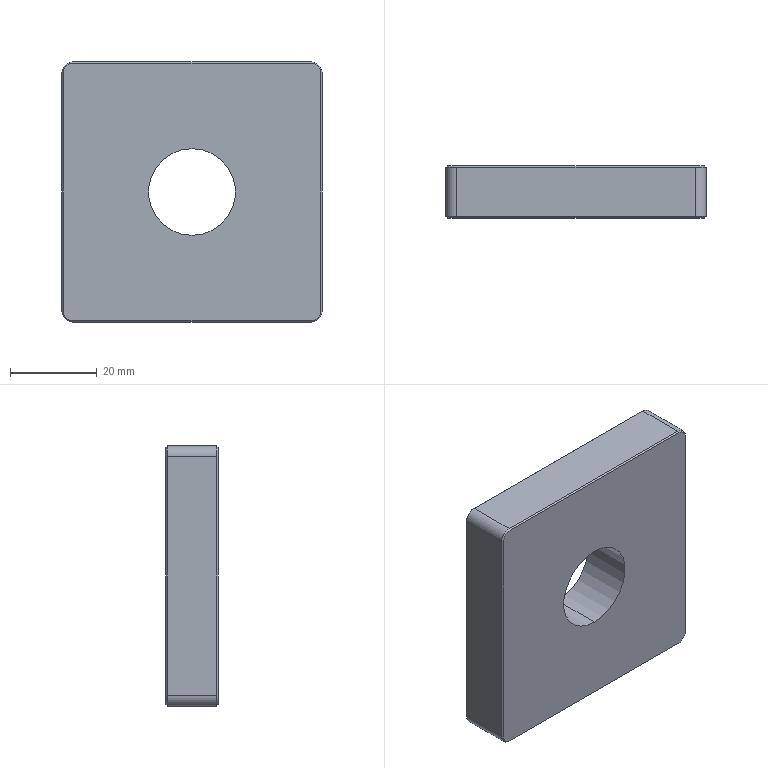Part | SolidWorks | features BaseBody 1 | 1 solid | 28 faces | box 60 x 12 x 60 mm | volume 39345 mm3 | plane 14 | cone 8 | cylinder 6 | commonest cylinder face diameters 5 x4 20 x2
STEP:
#1=CARTESIAN_POINT('',(0.,6.,-10.));
#2=VERTEX_POINT('',#1);
#3=CARTESIAN_POINT('',(0.,6.,10.));
#4=VERTEX_POINT('',#3);
#5=CARTESIAN_POINT('',(0.,6.,0.));
#6=DIRECTION('',(0.,1.,0.));
#7=DIRECTION('',(0.,0.,-1.));
#8=AXIS2_PLACEMENT_3D('',#5,#6,#7);
#9=CIRCLE('',#8,10.);
#10=EDGE_CURVE('',#2,#4,#9,.T.);
#11=ORIENTED_EDGE('',*,*,#10,.T.);
#12=CARTESIAN_POINT('',(0.,-6.,10.));
#13=VERTEX_POINT('',#12);
#14=CARTESIAN_POINT('',(0.,6.,10.));
#15=DIRECTION('',(0.,-1.,0.));
#16=VECTOR('',#15,1000.);
#17=LINE('',#14,#16);
#18=EDGE_CURVE('',#4,#13,#17,.T.);
#19=ORIENTED_EDGE('',*,*,#18,.T.);
#20=CARTESIAN_POINT('',(0.,-6.,-10.));
#21=VERTEX_POINT('',#20);
#22=CARTESIAN_POINT('',(0.,-6.,0.));
#23=DIRECTION('',(0.,1.,0.));
#24=DIRECTION('',(0.,0.,-1.));
#25=AXIS2_PLACEMENT_3D('',#22,#23,#24);
#26=CIRCLE('',#25,10.);
#27=EDGE_CURVE('',#21,#13,#26,.T.);
#28=ORIENTED_EDGE('',*,*,#27,.F.);
#29=CARTESIAN_POINT('',(0.,6.,-10.));
#30=DIRECTION('',(0.,-1.,0.));
#31=VECTOR('',#30,1000.);
#32=LINE('',#29,#31);
#33=EDGE_CURVE('',#2,#21,#32,.T.);
#34=ORIENTED_EDGE('',*,*,#33,.F.);
#35=EDGE_LOOP('',(#11,#19,#28,#34));
#36=FACE_OUTER_BOUND('',#35,.T.);
#37=CARTESIAN_POINT('',(0.,6.,0.));
#38=DIRECTION('',(0.,-1.,0.));
#39=DIRECTION('',(0.,0.,-1.));
#40=AXIS2_PLACEMENT_3D('',#37,#38,#39);
#41=CYLINDRICAL_SURFACE('',#40,10.);
#42=ADVANCED_FACE('',(#36),#41,.F.);
#43=CARTESIAN_POINT('',(-27.5,6.,-29.7));
#44=VERTEX_POINT('',#43);
#45=CARTESIAN_POINT('',(27.5,6.,-29.7));
#46=VERTEX_POINT('',#45);
#47=CARTESIAN_POINT('',(0.,6.,-29.7));
#48=DIRECTION('',(1.,0.,0.));
#49=VECTOR('',#48,1000.);
#50=LINE('',#47,#49);
#51=EDGE_CURVE('',#44,#46,#50,.T.);
#52=ORIENTED_EDGE('',*,*,#51,.F.);
#53=CARTESIAN_POINT('',(-29.7,6.,-27.5));
#54=VERTEX_POINT('',#53);
#55=CARTESIAN_POINT('',(-27.5,6.,-27.5));
#56=DIRECTION('',(0.,-1.,0.));
#57=DIRECTION('',(0.,0.,-1.));
#58=AXIS2_PLACEMENT_3D('',#55,#56,#57);
#59=CIRCLE('',#58,2.2);
#60=EDGE_CURVE('',#54,#44,#59,.T.);
#61=ORIENTED_EDGE('',*,*,#60,.F.);
#62=CARTESIAN_POINT('',(-29.7,6.,27.5));
#63=VERTEX_POINT('',#62);
#64=CARTESIAN_POINT('',(-29.7,6.,0.));
#65=DIRECTION('',(0.,0.,-1.));
#66=VECTOR('',#65,1000.);
#67=LINE('',#64,#66);
#68=EDGE_CURVE('',#63,#54,#67,.T.);
#69=ORIENTED_EDGE('',*,*,#68,.F.);
#70=CARTESIAN_POINT('',(-27.5,6.,29.7));
#71=VERTEX_POINT('',#70);
#72=CARTESIAN_POINT('',(-27.5,6.,27.5));
#73=DIRECTION('',(0.,-1.,0.));
#74=DIRECTION('',(0.,0.,-1.));
#75=AXIS2_PLACEMENT_3D('',#72,#73,#74);
#76=CIRCLE('',#75,2.2);
#77=EDGE_CURVE('',#71,#63,#76,.T.);
#78=ORIENTED_EDGE('',*,*,#77,.F.);
#79=CARTESIAN_POINT('',(27.5,6.,29.7));
#80=VERTEX_POINT('',#79);
#81=CARTESIAN_POINT('',(0.,6.,29.7));
#82=DIRECTION('',(-1.,0.,0.));
#83=VECTOR('',#82,1000.);
#84=LINE('',#81,#83);
#85=EDGE_CURVE('',#80,#71,#84,.T.);
#86=ORIENTED_EDGE('',*,*,#85,.F.);
#87=CARTESIAN_POINT('',(29.7,6.,27.5));
#88=VERTEX_POINT('',#87);
#89=CARTESIAN_POINT('',(27.5,6.,27.5));
#90=DIRECTION('',(0.,-1.,0.));
#91=DIRECTION('',(0.,0.,-1.));
#92=AXIS2_PLACEMENT_3D('',#89,#90,#91);
#93=CIRCLE('',#92,2.2);
#94=EDGE_CURVE('',#88,#80,#93,.T.);
#95=ORIENTED_EDGE('',*,*,#94,.F.);
#96=CARTESIAN_POINT('',(29.7,6.,-27.5));
#97=VERTEX_POINT('',#96);
#98=CARTESIAN_POINT('',(29.7,6.,0.));
#99=DIRECTION('',(0.,0.,1.));
#100=VECTOR('',#99,1000.);
#101=LINE('',#98,#100);
#102=EDGE_CURVE('',#97,#88,#101,.T.);
#103=ORIENTED_EDGE('',*,*,#102,.F.);
#104=CARTESIAN_POINT('',(27.5,6.,-27.5));
#105=DIRECTION('',(0.,-1.,0.));
#106=DIRECTION('',(0.,0.,-1.));
#107=AXIS2_PLACEMENT_3D('',#104,#105,#106);
#108=CIRCLE('',#107,2.2);
#109=EDGE_CURVE('',#46,#97,#108,.T.);
#110=ORIENTED_EDGE('',*,*,#109,.F.);
#111=EDGE_LOOP('',(#52,#61,#69,#78,#86,#95,#103,#110));
#112=FACE_OUTER_BOUND('',#111,.T.);
#113=ORIENTED_EDGE('',*,*,#10,.F.);
#114=CARTESIAN_POINT('',(0.,6.,0.));
#115=DIRECTION('',(0.,1.,0.));
#116=DIRECTION('',(0.,0.,-1.));
#117=AXIS2_PLACEMENT_3D('',#114,#115,#116);
#118=CIRCLE('',#117,10.);
#119=EDGE_CURVE('',#4,#2,#118,.T.);
#120=ORIENTED_EDGE('',*,*,#119,.F.);
#121=EDGE_LOOP('',(#113,#120));
#122=FACE_BOUND('',#121,.T.);
#123=CARTESIAN_POINT('',(0.,6.,0.));
#124=DIRECTION('',(0.,-1.,0.));
#125=DIRECTION('',(0.,0.,-1.));
#126=AXIS2_PLACEMENT_3D('',#123,#124,#125);
#127=PLANE('',#126);
#128=ADVANCED_FACE('',(#112,#122),#127,.F.);
#129=CARTESIAN_POINT('',(27.5,5.7,-30.));
#130=VERTEX_POINT('',#129);
#131=CARTESIAN_POINT('',(27.5,-498964.3,-499000.));
#132=DIRECTION('',(0.,0.7071,0.7071));
#133=VECTOR('',#132,1000.);
#134=LINE('',#131,#133);
#135=EDGE_CURVE('',#130,#46,#134,.T.);
#136=ORIENTED_EDGE('',*,*,#135,.T.);
#137=ORIENTED_EDGE('',*,*,#109,.T.);
#138=CARTESIAN_POINT('',(30.,5.7,-27.5));
#139=VERTEX_POINT('',#138);
#140=CARTESIAN_POINT('',(499000.,-498964.3,-27.5));
#141=DIRECTION('',(0.7071,-0.7071,0.));
#142=VECTOR('',#141,1000.);
#143=LINE('',#140,#142);
#144=EDGE_CURVE('',#97,#139,#143,.T.);
#145=ORIENTED_EDGE('',*,*,#144,.T.);
#146=CARTESIAN_POINT('',(27.5,5.7,-27.5));
#147=DIRECTION('',(0.,1.,0.));
#148=DIRECTION('',(0.,0.,-1.));
#149=AXIS2_PLACEMENT_3D('',#146,#147,#148);
#150=CIRCLE('',#149,2.5);
#151=EDGE_CURVE('',#139,#130,#150,.T.);
#152=ORIENTED_EDGE('',*,*,#151,.T.);
#153=EDGE_LOOP('',(#136,#137,#145,#152));
#154=FACE_OUTER_BOUND('',#153,.T.);
#155=CARTESIAN_POINT('',(27.5,5.7,-27.5));
#156=DIRECTION('',(0.,-1.,0.));
#157=DIRECTION('',(0.,0.,-1.));
#158=AXIS2_PLACEMENT_3D('',#155,#156,#157);
#159=CONICAL_SURFACE('',#158,2.5,0.7854);
#160=ADVANCED_FACE('',(#154),#159,.T.);
#161=CARTESIAN_POINT('',(-27.5,5.7,-30.));
#162=VERTEX_POINT('',#161);
#163=CARTESIAN_POINT('',(0.,5.7,-30.));
#164=DIRECTION('',(1.,0.,0.));
#165=VECTOR('',#164,1000.);
#166=LINE('',#163,#165);
#167=EDGE_CURVE('',#162,#130,#166,.T.);
#168=ORIENTED_EDGE('',*,*,#167,.F.);
#169=CARTESIAN_POINT('',(-27.5,6.,-29.7));
#170=DIRECTION('',(0.,-0.7071,-0.7071));
#171=VECTOR('',#170,1000.);
#172=LINE('',#169,#171);
#173=EDGE_CURVE('',#44,#162,#172,.T.);
#174=ORIENTED_EDGE('',*,*,#173,.F.);
#175=ORIENTED_EDGE('',*,*,#51,.T.);
#176=ORIENTED_EDGE('',*,*,#135,.F.);
#177=EDGE_LOOP('',(#168,#174,#175,#176));
#178=FACE_OUTER_BOUND('',#177,.T.);
#179=CARTESIAN_POINT('',(0.,6.,-29.7));
#180=DIRECTION('',(0.,-0.7071,0.7071));
#181=DIRECTION('',(0.,-0.7071,-0.7071));
#182=AXIS2_PLACEMENT_3D('',#179,#180,#181);
#183=PLANE('',#182);
#184=ADVANCED_FACE('',(#178),#183,.F.);
#185=ORIENTED_EDGE('',*,*,#173,.T.);
#186=CARTESIAN_POINT('',(-30.,5.7,-27.5));
#187=VERTEX_POINT('',#186);
#188=CARTESIAN_POINT('',(-27.5,5.7,-27.5));
#189=DIRECTION('',(0.,1.,0.));
#190=DIRECTION('',(0.,0.,-1.));
#191=AXIS2_PLACEMENT_3D('',#188,#189,#190);
#192=CIRCLE('',#191,2.5);
#193=EDGE_CURVE('',#162,#187,#192,.T.);
#194=ORIENTED_EDGE('',*,*,#193,.T.);
#195=CARTESIAN_POINT('',(-499000.,-498964.3,-27.5));
#196=DIRECTION('',(0.7071,0.7071,0.));
#197=VECTOR('',#196,1000.);
#198=LINE('',#195,#197);
#199=EDGE_CURVE('',#187,#54,#198,.T.);
#200=ORIENTED_EDGE('',*,*,#199,.T.);
#201=ORIENTED_EDGE('',*,*,#60,.T.);
#202=EDGE_LOOP('',(#185,#194,#200,#201));
#203=FACE_OUTER_BOUND('',#202,.T.);
#204=CARTESIAN_POINT('',(-27.5,5.7,-27.5));
#205=DIRECTION('',(0.,-1.,0.));
#206=DIRECTION('',(0.,0.,-1.));
#207=AXIS2_PLACEMENT_3D('',#204,#205,#206);
#208=CONICAL_SURFACE('',#207,2.5,0.7854);
#209=ADVANCED_FACE('',(#203),#208,.T.);
#210=ORIENTED_EDGE('',*,*,#68,.T.);
#211=ORIENTED_EDGE('',*,*,#199,.F.);
#212=CARTESIAN_POINT('',(-30.,5.7,27.5));
#213=VERTEX_POINT('',#212);
#214=CARTESIAN_POINT('',(-30.,5.7,0.));
#215=DIRECTION('',(0.,0.,-1.));
#216=VECTOR('',#215,1000.);
#217=LINE('',#214,#216);
#218=EDGE_CURVE('',#213,#187,#217,.T.);
#219=ORIENTED_EDGE('',*,*,#218,.F.);
#220=CARTESIAN_POINT('',(-29.7,6.,27.5));
#221=DIRECTION('',(-0.7071,-0.7071,0.));
#222=VECTOR('',#221,1000.);
#223=LINE('',#220,#222);
#224=EDGE_CURVE('',#63,#213,#223,.T.);
#225=ORIENTED_EDGE('',*,*,#224,.F.);
#226=EDGE_LOOP('',(#210,#211,#219,#225));
#227=FACE_OUTER_BOUND('',#226,.T.);
#228=CARTESIAN_POINT('',(-29.7,6.,0.));
#229=DIRECTION('',(0.7071,-0.7071,0.));
#230=DIRECTION('',(0.7071,0.7071,0.));
#231=AXIS2_PLACEMENT_3D('',#228,#229,#230);
#232=PLANE('',#231);
#233=ADVANCED_FACE('',(#227),#232,.F.);
#234=ORIENTED_EDGE('',*,*,#224,.T.);
#235=CARTESIAN_POINT('',(-27.5,5.7,30.));
#236=VERTEX_POINT('',#235);
#237=CARTESIAN_POINT('',(-27.5,5.7,27.5));
#238=DIRECTION('',(0.,1.,0.));
#239=DIRECTION('',(0.,0.,-1.));
#240=AXIS2_PLACEMENT_3D('',#237,#238,#239);
#241=CIRCLE('',#240,2.5);
#242=EDGE_CURVE('',#213,#236,#241,.T.);
#243=ORIENTED_EDGE('',*,*,#242,.T.);
#244=CARTESIAN_POINT('',(-27.5,-499000.,499035.7));
#245=DIRECTION('',(0.,0.7071,-0.7071));
#246=VECTOR('',#245,1000.);
#247=LINE('',#244,#246);
#248=EDGE_CURVE('',#236,#71,#247,.T.);
#249=ORIENTED_EDGE('',*,*,#248,.T.);
#250=ORIENTED_EDGE('',*,*,#77,.T.);
#251=EDGE_LOOP('',(#234,#243,#249,#250));
#252=FACE_OUTER_BOUND('',#251,.T.);
#253=CARTESIAN_POINT('',(-27.5,5.7,27.5));
#254=DIRECTION('',(0.,-1.,0.));
#255=DIRECTION('',(0.,0.,-1.));
#256=AXIS2_PLACEMENT_3D('',#253,#254,#255);
#257=CONICAL_SURFACE('',#256,2.5,0.7854);
#258=ADVANCED_FACE('',(#252),#257,.T.);
#259=CARTESIAN_POINT('',(27.5,5.7,30.));
#260=VERTEX_POINT('',#259);
#261=CARTESIAN_POINT('',(0.,5.7,30.));
#262=DIRECTION('',(-1.,0.,0.));
#263=VECTOR('',#262,1000.);
#264=LINE('',#261,#263);
#265=EDGE_CURVE('',#260,#236,#264,.T.);
#266=ORIENTED_EDGE('',*,*,#265,.F.);
#267=CARTESIAN_POINT('',(27.5,6.,29.7));
#268=DIRECTION('',(0.,-0.7071,0.7071));
#269=VECTOR('',#268,1000.);
#270=LINE('',#267,#269);
#271=EDGE_CURVE('',#80,#260,#270,.T.);
#272=ORIENTED_EDGE('',*,*,#271,.F.);
#273=ORIENTED_EDGE('',*,*,#85,.T.);
#274=ORIENTED_EDGE('',*,*,#248,.F.);
#275=EDGE_LOOP('',(#266,#272,#273,#274));
#276=FACE_OUTER_BOUND('',#275,.T.);
#277=CARTESIAN_POINT('',(0.,6.,29.7));
#278=DIRECTION('',(0.,-0.7071,-0.7071));
#279=DIRECTION('',(0.,0.7071,-0.7071));
#280=AXIS2_PLACEMENT_3D('',#277,#278,#279);
#281=PLANE('',#280);
#282=ADVANCED_FACE('',(#276),#281,.F.);
#283=CARTESIAN_POINT('',(30.,5.7,27.5));
#284=VERTEX_POINT('',#283);
#285=CARTESIAN_POINT('',(499035.7,-499000.,27.5));
#286=DIRECTION('',(-0.7071,0.7071,0.));
#287=VECTOR('',#286,1000.);
#288=LINE('',#285,#287);
#289=EDGE_CURVE('',#284,#88,#288,.T.);
#290=ORIENTED_EDGE('',*,*,#289,.T.);
#291=ORIENTED_EDGE('',*,*,#94,.T.);
#292=ORIENTED_EDGE('',*,*,#271,.T.);
#293=CARTESIAN_POINT('',(27.5,5.7,27.5));
#294=DIRECTION('',(0.,1.,0.));
#295=DIRECTION('',(0.,0.,-1.));
#296=AXIS2_PLACEMENT_3D('',#293,#294,#295);
#297=CIRCLE('',#296,2.5);
#298=EDGE_CURVE('',#260,#284,#297,.T.);
#299=ORIENTED_EDGE('',*,*,#298,.T.);
#300=EDGE_LOOP('',(#290,#291,#292,#299));
#301=FACE_OUTER_BOUND('',#300,.T.);
#302=CARTESIAN_POINT('',(27.5,5.7,27.5));
#303=DIRECTION('',(0.,-1.,0.));
#304=DIRECTION('',(0.,0.,-1.));
#305=AXIS2_PLACEMENT_3D('',#302,#303,#304);
#306=CONICAL_SURFACE('',#305,2.5,0.7854);
#307=ADVANCED_FACE('',(#301),#306,.T.);
#308=CARTESIAN_POINT('',(30.,5.7,0.));
#309=DIRECTION('',(0.,0.,1.));
#310=VECTOR('',#309,1000.);
#311=LINE('',#308,#310);
#312=EDGE_CURVE('',#139,#284,#311,.T.);
#313=ORIENTED_EDGE('',*,*,#312,.F.);
#314=ORIENTED_EDGE('',*,*,#144,.F.);
#315=ORIENTED_EDGE('',*,*,#102,.T.);
#316=ORIENTED_EDGE('',*,*,#289,.F.);
#317=EDGE_LOOP('',(#313,#314,#315,#316));
#318=FACE_OUTER_BOUND('',#317,.T.);
#319=CARTESIAN_POINT('',(29.7,6.,0.));
#320=DIRECTION('',(-0.7071,-0.7071,0.));
#321=DIRECTION('',(0.7071,-0.7071,0.));
#322=AXIS2_PLACEMENT_3D('',#319,#320,#321);
#323=PLANE('',#322);
#324=ADVANCED_FACE('',(#318),#323,.F.);
#325=ORIENTED_EDGE('',*,*,#18,.F.);
#326=ORIENTED_EDGE('',*,*,#119,.T.);
#327=ORIENTED_EDGE('',*,*,#33,.T.);
#328=CARTESIAN_POINT('',(0.,-6.,0.));
#329=DIRECTION('',(0.,1.,0.));
#330=DIRECTION('',(0.,0.,-1.));
#331=AXIS2_PLACEMENT_3D('',#328,#329,#330);
#332=CIRCLE('',#331,10.);
#333=EDGE_CURVE('',#13,#21,#332,.T.);
#334=ORIENTED_EDGE('',*,*,#333,.F.);
#335=EDGE_LOOP('',(#325,#326,#327,#334));
#336=FACE_OUTER_BOUND('',#335,.T.);
#337=CARTESIAN_POINT('',(0.,6.,0.));
#338=DIRECTION('',(0.,-1.,0.));
#339=DIRECTION('',(0.,0.,-1.));
#340=AXIS2_PLACEMENT_3D('',#337,#338,#339);
#341=CYLINDRICAL_SURFACE('',#340,10.);
#342=ADVANCED_FACE('',(#336),#341,.F.);
#343=CARTESIAN_POINT('',(27.5,-5.7,-30.));
#344=VERTEX_POINT('',#343);
#345=CARTESIAN_POINT('',(27.5,6.,-30.));
#346=DIRECTION('',(0.,1.,0.));
#347=VECTOR('',#346,1000.);
#348=LINE('',#345,#347);
#349=EDGE_CURVE('',#344,#130,#348,.T.);
#350=ORIENTED_EDGE('',*,*,#349,.T.);
#351=ORIENTED_EDGE('',*,*,#151,.F.);
#352=CARTESIAN_POINT('',(30.,-5.7,-27.5));
#353=VERTEX_POINT('',#352);
#354=CARTESIAN_POINT('',(30.,6.,-27.5));
#355=DIRECTION('',(0.,-1.,0.));
#356=VECTOR('',#355,1000.);
#357=LINE('',#354,#356);
#358=EDGE_CURVE('',#139,#353,#357,.T.);
#359=ORIENTED_EDGE('',*,*,#358,.T.);
#360=CARTESIAN_POINT('',(27.5,-5.7,-27.5));
#361=DIRECTION('',(0.,1.,0.));
#362=DIRECTION('',(0.,0.,-1.));
#363=AXIS2_PLACEMENT_3D('',#360,#361,#362);
#364=CIRCLE('',#363,2.5);
#365=EDGE_CURVE('',#353,#344,#364,.T.);
#366=ORIENTED_EDGE('',*,*,#365,.T.);
#367=EDGE_LOOP('',(#350,#351,#359,#366));
#368=FACE_OUTER_BOUND('',#367,.T.);
#369=CARTESIAN_POINT('',(27.5,6.,-27.5));
#370=DIRECTION('',(0.,-1.,0.));
#371=DIRECTION('',(0.,0.,-1.));
#372=AXIS2_PLACEMENT_3D('',#369,#370,#371);
#373=CYLINDRICAL_SURFACE('',#372,2.5);
#374=ADVANCED_FACE('',(#368),#373,.T.);
#375=ORIENTED_EDGE('',*,*,#167,.T.);
#376=ORIENTED_EDGE('',*,*,#349,.F.);
#377=CARTESIAN_POINT('',(-27.5,-5.7,-30.));
#378=VERTEX_POINT('',#377);
#379=CARTESIAN_POINT('',(30.,-5.7,-30.));
#380=DIRECTION('',(1.,0.,0.));
#381=VECTOR('',#380,1000.);
#382=LINE('',#379,#381);
#383=EDGE_CURVE('',#378,#344,#382,.T.);
#384=ORIENTED_EDGE('',*,*,#383,.F.);
#385=CARTESIAN_POINT('',(-27.5,6.,-30.));
#386=DIRECTION('',(0.,-1.,0.));
#387=VECTOR('',#386,1000.);
#388=LINE('',#385,#387);
#389=EDGE_CURVE('',#162,#378,#388,.T.);
#390=ORIENTED_EDGE('',*,*,#389,.F.);
#391=EDGE_LOOP('',(#375,#376,#384,#390));
#392=FACE_OUTER_BOUND('',#391,.T.);
#393=CARTESIAN_POINT('',(30.,6.,-30.));
#394=DIRECTION('',(0.,0.,1.));
#395=DIRECTION('',(1.,0.,0.));
#396=AXIS2_PLACEMENT_3D('',#393,#394,#395);
#397=PLANE('',#396);
#398=ADVANCED_FACE('',(#392),#397,.F.);
#399=CARTESIAN_POINT('',(-30.,-5.7,-27.5));
#400=VERTEX_POINT('',#399);
#401=CARTESIAN_POINT('',(-30.,6.,-27.5));
#402=DIRECTION('',(0.,1.,0.));
#403=VECTOR('',#402,1000.);
#404=LINE('',#401,#403);
#405=EDGE_CURVE('',#400,#187,#404,.T.);
#406=ORIENTED_EDGE('',*,*,#405,.T.);
#407=ORIENTED_EDGE('',*,*,#193,.F.);
#408=ORIENTED_EDGE('',*,*,#389,.T.);
#409=CARTESIAN_POINT('',(-27.5,-5.7,-27.5));
#410=DIRECTION('',(0.,1.,0.));
#411=DIRECTION('',(0.,0.,-1.));
#412=AXIS2_PLACEMENT_3D('',#409,#410,#411);
#413=CIRCLE('',#412,2.5);
#414=EDGE_CURVE('',#378,#400,#413,.T.);
#415=ORIENTED_EDGE('',*,*,#414,.T.);
#416=EDGE_LOOP('',(#406,#407,#408,#415));
#417=FACE_OUTER_BOUND('',#416,.T.);
#418=CARTESIAN_POINT('',(-27.5,6.,-27.5));
#419=DIRECTION('',(0.,-1.,0.));
#420=DIRECTION('',(0.,0.,-1.));
#421=AXIS2_PLACEMENT_3D('',#418,#419,#420);
#422=CYLINDRICAL_SURFACE('',#421,2.5);
#423=ADVANCED_FACE('',(#417),#422,.T.);
#424=CARTESIAN_POINT('',(-30.,-5.7,27.5));
#425=VERTEX_POINT('',#424);
#426=CARTESIAN_POINT('',(-30.,-5.7,-30.));
#427=DIRECTION('',(0.,0.,-1.));
#428=VECTOR('',#427,1000.);
#429=LINE('',#426,#428);
#430=EDGE_CURVE('',#425,#400,#429,.T.);
#431=ORIENTED_EDGE('',*,*,#430,.F.);
#432=CARTESIAN_POINT('',(-30.,6.,27.5));
#433=DIRECTION('',(0.,-1.,0.));
#434=VECTOR('',#433,1000.);
#435=LINE('',#432,#434);
#436=EDGE_CURVE('',#213,#425,#435,.T.);
#437=ORIENTED_EDGE('',*,*,#436,.F.);
#438=ORIENTED_EDGE('',*,*,#218,.T.);
#439=ORIENTED_EDGE('',*,*,#405,.F.);
#440=EDGE_LOOP('',(#431,#437,#438,#439));
#441=FACE_OUTER_BOUND('',#440,.T.);
#442=CARTESIAN_POINT('',(-30.,6.,-30.));
#443=DIRECTION('',(1.,0.,0.));
#444=DIRECTION('',(0.,0.,-1.));
#445=AXIS2_PLACEMENT_3D('',#442,#443,#444);
#446=PLANE('',#445);
#447=ADVANCED_FACE('',(#441),#446,.F.);
#448=CARTESIAN_POINT('',(-27.5,-5.7,30.));
#449=VERTEX_POINT('',#448);
#450=CARTESIAN_POINT('',(-27.5,6.,30.));
#451=DIRECTION('',(0.,1.,0.));
#452=VECTOR('',#451,1000.);
#453=LINE('',#450,#452);
#454=EDGE_CURVE('',#449,#236,#453,.T.);
#455=ORIENTED_EDGE('',*,*,#454,.T.);
#456=ORIENTED_EDGE('',*,*,#242,.F.);
#457=ORIENTED_EDGE('',*,*,#436,.T.);
#458=CARTESIAN_POINT('',(-27.5,-5.7,27.5));
#459=DIRECTION('',(0.,1.,0.));
#460=DIRECTION('',(0.,0.,-1.));
#461=AXIS2_PLACEMENT_3D('',#458,#459,#460);
#462=CIRCLE('',#461,2.5);
#463=EDGE_CURVE('',#425,#449,#462,.T.);
#464=ORIENTED_EDGE('',*,*,#463,.T.);
#465=EDGE_LOOP('',(#455,#456,#457,#464));
#466=FACE_OUTER_BOUND('',#465,.T.);
#467=CARTESIAN_POINT('',(-27.5,6.,27.5));
#468=DIRECTION('',(0.,-1.,0.));
#469=DIRECTION('',(0.,0.,-1.));
#470=AXIS2_PLACEMENT_3D('',#467,#468,#469);
#471=CYLINDRICAL_SURFACE('',#470,2.5);
#472=ADVANCED_FACE('',(#466),#471,.T.);
#473=CARTESIAN_POINT('',(27.5,-5.7,30.));
#474=VERTEX_POINT('',#473);
#475=CARTESIAN_POINT('',(30.,-5.7,30.));
#476=DIRECTION('',(-1.,0.,0.));
#477=VECTOR('',#476,1000.);
#478=LINE('',#475,#477);
#479=EDGE_CURVE('',#474,#449,#478,.T.);
#480=ORIENTED_EDGE('',*,*,#479,.F.);
#481=CARTESIAN_POINT('',(27.5,6.,30.));
#482=DIRECTION('',(0.,-1.,0.));
#483=VECTOR('',#482,1000.);
#484=LINE('',#481,#483);
#485=EDGE_CURVE('',#260,#474,#484,.T.);
#486=ORIENTED_EDGE('',*,*,#485,.F.);
#487=ORIENTED_EDGE('',*,*,#265,.T.);
#488=ORIENTED_EDGE('',*,*,#454,.F.);
#489=EDGE_LOOP('',(#480,#486,#487,#488));
#490=FACE_OUTER_BOUND('',#489,.T.);
#491=CARTESIAN_POINT('',(30.,6.,30.));
#492=DIRECTION('',(0.,0.,-1.));
#493=DIRECTION('',(-1.,0.,0.));
#494=AXIS2_PLACEMENT_3D('',#491,#492,#493);
#495=PLANE('',#494);
#496=ADVANCED_FACE('',(#490),#495,.F.);
#497=CARTESIAN_POINT('',(30.,-5.7,27.5));
#498=VERTEX_POINT('',#497);
#499=CARTESIAN_POINT('',(30.,6.,27.5));
#500=DIRECTION('',(0.,1.,0.));
#501=VECTOR('',#500,1000.);
#502=LINE('',#499,#501);
#503=EDGE_CURVE('',#498,#284,#502,.T.);
#504=ORIENTED_EDGE('',*,*,#503,.T.);
#505=ORIENTED_EDGE('',*,*,#298,.F.);
#506=ORIENTED_EDGE('',*,*,#485,.T.);
#507=CARTESIAN_POINT('',(27.5,-5.7,27.5));
#508=DIRECTION('',(0.,1.,0.));
#509=DIRECTION('',(0.,0.,-1.));
#510=AXIS2_PLACEMENT_3D('',#507,#508,#509);
#511=CIRCLE('',#510,2.5);
#512=EDGE_CURVE('',#474,#498,#511,.T.);
#513=ORIENTED_EDGE('',*,*,#512,.T.);
#514=EDGE_LOOP('',(#504,#505,#506,#513));
#515=FACE_OUTER_BOUND('',#514,.T.);
#516=CARTESIAN_POINT('',(27.5,6.,27.5));
#517=DIRECTION('',(0.,-1.,0.));
#518=DIRECTION('',(0.,0.,-1.));
#519=AXIS2_PLACEMENT_3D('',#516,#517,#518);
#520=CYLINDRICAL_SURFACE('',#519,2.5);
#521=ADVANCED_FACE('',(#515),#520,.T.);
#522=CARTESIAN_POINT('',(30.,-5.7,-30.));
#523=DIRECTION('',(0.,0.,1.));
#524=VECTOR('',#523,1000.);
#525=LINE('',#522,#524);
#526=EDGE_CURVE('',#353,#498,#525,.T.);
#527=ORIENTED_EDGE('',*,*,#526,.F.);
#528=ORIENTED_EDGE('',*,*,#358,.F.);
#529=ORIENTED_EDGE('',*,*,#312,.T.);
#530=ORIENTED_EDGE('',*,*,#503,.F.);
#531=EDGE_LOOP('',(#527,#528,#529,#530));
#532=FACE_OUTER_BOUND('',#531,.T.);
#533=CARTESIAN_POINT('',(30.,6.,-30.));
#534=DIRECTION('',(-1.,0.,0.));
#535=DIRECTION('',(0.,0.,1.));
#536=AXIS2_PLACEMENT_3D('',#533,#534,#535);
#537=PLANE('',#536);
#538=ADVANCED_FACE('',(#532),#537,.F.);
#539=CARTESIAN_POINT('',(-29.7,-6.,27.5));
#540=VERTEX_POINT('',#539);
#541=CARTESIAN_POINT('',(-29.7,-6.,-27.5));
#542=VERTEX_POINT('',#541);
#543=CARTESIAN_POINT('',(-29.7,-6.,0.));
#544=DIRECTION('',(0.,0.,-1.));
#545=VECTOR('',#544,1000.);
#546=LINE('',#543,#545);
#547=EDGE_CURVE('',#540,#542,#546,.T.);
#548=ORIENTED_EDGE('',*,*,#547,.T.);
#549=CARTESIAN_POINT('',(-27.5,-6.,-29.7));
#550=VERTEX_POINT('',#549);
#551=CARTESIAN_POINT('',(-27.5,-6.,-27.5));
#552=DIRECTION('',(0.,-1.,0.));
#553=DIRECTION('',(0.,0.,1.));
#554=AXIS2_PLACEMENT_3D('',#551,#552,#553);
#555=CIRCLE('',#554,2.2);
#556=EDGE_CURVE('',#542,#550,#555,.T.);
#557=ORIENTED_EDGE('',*,*,#556,.T.);
#558=CARTESIAN_POINT('',(27.5,-6.,-29.7));
#559=VERTEX_POINT('',#558);
#560=CARTESIAN_POINT('',(0.,-6.,-29.7));
#561=DIRECTION('',(1.,0.,0.));
#562=VECTOR('',#561,1000.);
#563=LINE('',#560,#562);
#564=EDGE_CURVE('',#550,#559,#563,.T.);
#565=ORIENTED_EDGE('',*,*,#564,.T.);
#566=CARTESIAN_POINT('',(29.7,-6.,-27.5));
#567=VERTEX_POINT('',#566);
#568=CARTESIAN_POINT('',(27.5,-6.,-27.5));
#569=DIRECTION('',(0.,-1.,0.));
#570=DIRECTION('',(0.,0.,1.));
#571=AXIS2_PLACEMENT_3D('',#568,#569,#570);
#572=CIRCLE('',#571,2.2);
#573=EDGE_CURVE('',#559,#567,#572,.T.);
#574=ORIENTED_EDGE('',*,*,#573,.T.);
#575=CARTESIAN_POINT('',(29.7,-6.,27.5));
#576=VERTEX_POINT('',#575);
#577=CARTESIAN_POINT('',(29.7,-6.,0.));
#578=DIRECTION('',(0.,0.,1.));
#579=VECTOR('',#578,1000.);
#580=LINE('',#577,#579);
#581=EDGE_CURVE('',#567,#576,#580,.T.);
#582=ORIENTED_EDGE('',*,*,#581,.T.);
#583=CARTESIAN_POINT('',(27.5,-6.,29.7));
#584=VERTEX_POINT('',#583);
#585=CARTESIAN_POINT('',(27.5,-6.,27.5));
#586=DIRECTION('',(0.,-1.,0.));
#587=DIRECTION('',(0.,0.,1.));
#588=AXIS2_PLACEMENT_3D('',#585,#586,#587);
#589=CIRCLE('',#588,2.2);
#590=EDGE_CURVE('',#576,#584,#589,.T.);
#591=ORIENTED_EDGE('',*,*,#590,.T.);
#592=CARTESIAN_POINT('',(-27.5,-6.,29.7));
#593=VERTEX_POINT('',#592);
#594=CARTESIAN_POINT('',(0.,-6.,29.7));
#595=DIRECTION('',(-1.,0.,0.));
#596=VECTOR('',#595,1000.);
#597=LINE('',#594,#596);
#598=EDGE_CURVE('',#584,#593,#597,.T.);
#599=ORIENTED_EDGE('',*,*,#598,.T.);
#600=CARTESIAN_POINT('',(-27.5,-6.,27.5));
#601=DIRECTION('',(0.,-1.,0.));
#602=DIRECTION('',(0.,0.,1.));
#603=AXIS2_PLACEMENT_3D('',#600,#601,#602);
#604=CIRCLE('',#603,2.2);
#605=EDGE_CURVE('',#593,#540,#604,.T.);
#606=ORIENTED_EDGE('',*,*,#605,.T.);
#607=EDGE_LOOP('',(#548,#557,#565,#574,#582,#591,#599,#606));
#608=FACE_OUTER_BOUND('',#607,.T.);
#609=ORIENTED_EDGE('',*,*,#27,.T.);
#610=ORIENTED_EDGE('',*,*,#333,.T.);
#611=EDGE_LOOP('',(#609,#610));
#612=FACE_BOUND('',#611,.T.);
#613=CARTESIAN_POINT('',(0.,-6.,0.));
#614=DIRECTION('',(0.,-1.,0.));
#615=DIRECTION('',(0.,0.,-1.));
#616=AXIS2_PLACEMENT_3D('',#613,#614,#615);
#617=PLANE('',#616);
#618=ADVANCED_FACE('',(#608,#612),#617,.T.);
#619=CARTESIAN_POINT('',(27.5,499000.,-499035.7));
#620=DIRECTION('',(0.,0.7071,-0.7071));
#621=VECTOR('',#620,1000.);
#622=LINE('',#619,#621);
#623=EDGE_CURVE('',#559,#344,#622,.T.);
#624=ORIENTED_EDGE('',*,*,#623,.T.);
#625=ORIENTED_EDGE('',*,*,#365,.F.);
#626=CARTESIAN_POINT('',(499035.7,499000.,-27.5));
#627=DIRECTION('',(-0.7071,-0.7071,0.));
#628=VECTOR('',#627,1000.);
#629=LINE('',#626,#628);
#630=EDGE_CURVE('',#353,#567,#629,.T.);
#631=ORIENTED_EDGE('',*,*,#630,.T.);
#632=ORIENTED_EDGE('',*,*,#573,.F.);
#633=EDGE_LOOP('',(#624,#625,#631,#632));
#634=FACE_OUTER_BOUND('',#633,.T.);
#635=CARTESIAN_POINT('',(27.5,-5.7,-27.5));
#636=DIRECTION('',(0.,1.,0.));
#637=DIRECTION('',(0.,0.,1.));
#638=AXIS2_PLACEMENT_3D('',#635,#636,#637);
#639=CONICAL_SURFACE('',#638,2.5,0.7854);
#640=ADVANCED_FACE('',(#634),#639,.T.);
#641=CARTESIAN_POINT('',(-27.5,-5.7,-30.));
#642=DIRECTION('',(0.,0.7071,-0.7071));
#643=VECTOR('',#642,1000.);
#644=LINE('',#641,#643);
#645=EDGE_CURVE('',#550,#378,#644,.T.);
#646=ORIENTED_EDGE('',*,*,#645,.T.);
#647=ORIENTED_EDGE('',*,*,#383,.T.);
#648=ORIENTED_EDGE('',*,*,#623,.F.);
#649=ORIENTED_EDGE('',*,*,#564,.F.);
#650=EDGE_LOOP('',(#646,#647,#648,#649));
#651=FACE_OUTER_BOUND('',#650,.T.);
#652=CARTESIAN_POINT('',(30.,-5.7,-30.));
#653=DIRECTION('',(0.,-0.7071,-0.7071));
#654=DIRECTION('',(0.,0.7071,-0.7071));
#655=AXIS2_PLACEMENT_3D('',#652,#653,#654);
#656=PLANE('',#655);
#657=ADVANCED_FACE('',(#651),#656,.T.);
#658=ORIENTED_EDGE('',*,*,#645,.F.);
#659=ORIENTED_EDGE('',*,*,#556,.F.);
#660=CARTESIAN_POINT('',(-499035.7,499000.,-27.5));
#661=DIRECTION('',(-0.7071,0.7071,0.));
#662=VECTOR('',#661,1000.);
#663=LINE('',#660,#662);
#664=EDGE_CURVE('',#542,#400,#663,.T.);
#665=ORIENTED_EDGE('',*,*,#664,.T.);
#666=ORIENTED_EDGE('',*,*,#414,.F.);
#667=EDGE_LOOP('',(#658,#659,#665,#666));
#668=FACE_OUTER_BOUND('',#667,.T.);
#669=CARTESIAN_POINT('',(-27.5,-5.7,-27.5));
#670=DIRECTION('',(0.,1.,0.));
#671=DIRECTION('',(0.,0.,1.));
#672=AXIS2_PLACEMENT_3D('',#669,#670,#671);
#673=CONICAL_SURFACE('',#672,2.5,0.7854);
#674=ADVANCED_FACE('',(#668),#673,.T.);
#675=ORIENTED_EDGE('',*,*,#664,.F.);
#676=ORIENTED_EDGE('',*,*,#547,.F.);
#677=CARTESIAN_POINT('',(-30.,-5.7,27.5));
#678=DIRECTION('',(-0.7071,0.7071,0.));
#679=VECTOR('',#678,1000.);
#680=LINE('',#677,#679);
#681=EDGE_CURVE('',#540,#425,#680,.T.);
#682=ORIENTED_EDGE('',*,*,#681,.T.);
#683=ORIENTED_EDGE('',*,*,#430,.T.);
#684=EDGE_LOOP('',(#675,#676,#682,#683));
#685=FACE_OUTER_BOUND('',#684,.T.);
#686=CARTESIAN_POINT('',(-30.,-5.7,-30.));
#687=DIRECTION('',(-0.7071,-0.7071,0.));
#688=DIRECTION('',(0.7071,-0.7071,0.));
#689=AXIS2_PLACEMENT_3D('',#686,#687,#688);
#690=PLANE('',#689);
#691=ADVANCED_FACE('',(#685),#690,.T.);
#692=ORIENTED_EDGE('',*,*,#681,.F.);
#693=ORIENTED_EDGE('',*,*,#605,.F.);
#694=CARTESIAN_POINT('',(-27.5,498964.3,499000.));
#695=DIRECTION('',(0.,0.7071,0.7071));
#696=VECTOR('',#695,1000.);
#697=LINE('',#694,#696);
#698=EDGE_CURVE('',#593,#449,#697,.T.);
#699=ORIENTED_EDGE('',*,*,#698,.T.);
#700=ORIENTED_EDGE('',*,*,#463,.F.);
#701=EDGE_LOOP('',(#692,#693,#699,#700));
#702=FACE_OUTER_BOUND('',#701,.T.);
#703=CARTESIAN_POINT('',(-27.5,-5.7,27.5));
#704=DIRECTION('',(0.,1.,0.));
#705=DIRECTION('',(0.,0.,1.));
#706=AXIS2_PLACEMENT_3D('',#703,#704,#705);
#707=CONICAL_SURFACE('',#706,2.5,0.7854);
#708=ADVANCED_FACE('',(#702),#707,.T.);
#709=CARTESIAN_POINT('',(27.5,-5.7,30.));
#710=DIRECTION('',(0.,0.7071,0.7071));
#711=VECTOR('',#710,1000.);
#712=LINE('',#709,#711);
#713=EDGE_CURVE('',#584,#474,#712,.T.);
#714=ORIENTED_EDGE('',*,*,#713,.T.);
#715=ORIENTED_EDGE('',*,*,#479,.T.);
#716=ORIENTED_EDGE('',*,*,#698,.F.);
#717=ORIENTED_EDGE('',*,*,#598,.F.);
#718=EDGE_LOOP('',(#714,#715,#716,#717));
#719=FACE_OUTER_BOUND('',#718,.T.);
#720=CARTESIAN_POINT('',(30.,-5.7,30.));
#721=DIRECTION('',(0.,-0.7071,0.7071));
#722=DIRECTION('',(0.,-0.7071,-0.7071));
#723=AXIS2_PLACEMENT_3D('',#720,#721,#722);
#724=PLANE('',#723);
#725=ADVANCED_FACE('',(#719),#724,.T.);
#726=CARTESIAN_POINT('',(499000.,498964.3,27.5));
#727=DIRECTION('',(0.7071,0.7071,0.));
#728=VECTOR('',#727,1000.);
#729=LINE('',#726,#728);
#730=EDGE_CURVE('',#576,#498,#729,.T.);
#731=ORIENTED_EDGE('',*,*,#730,.T.);
#732=ORIENTED_EDGE('',*,*,#512,.F.);
#733=ORIENTED_EDGE('',*,*,#713,.F.);
#734=ORIENTED_EDGE('',*,*,#590,.F.);
#735=EDGE_LOOP('',(#731,#732,#733,#734));
#736=FACE_OUTER_BOUND('',#735,.T.);
#737=CARTESIAN_POINT('',(27.5,-5.7,27.5));
#738=DIRECTION('',(0.,1.,0.));
#739=DIRECTION('',(0.,0.,1.));
#740=AXIS2_PLACEMENT_3D('',#737,#738,#739);
#741=CONICAL_SURFACE('',#740,2.5,0.7854);
#742=ADVANCED_FACE('',(#736),#741,.T.);
#743=ORIENTED_EDGE('',*,*,#630,.F.);
#744=ORIENTED_EDGE('',*,*,#526,.T.);
#745=ORIENTED_EDGE('',*,*,#730,.F.);
#746=ORIENTED_EDGE('',*,*,#581,.F.);
#747=EDGE_LOOP('',(#743,#744,#745,#746));
#748=FACE_OUTER_BOUND('',#747,.T.);
#749=CARTESIAN_POINT('',(30.,-5.7,-30.));
#750=DIRECTION('',(0.7071,-0.7071,0.));
#751=DIRECTION('',(0.7071,0.7071,0.));
#752=AXIS2_PLACEMENT_3D('',#749,#750,#751);
#753=PLANE('',#752);
#754=ADVANCED_FACE('',(#748),#753,.T.);
#755=CLOSED_SHELL('',(#42,#128,#160,#184,#209,#233,#258,#282,#307,#324,#342,#374,#398,#423,#447,#472,#496,#521,#538,#618,#640,#657,#674,#691,#708,#725,#742,#754));
#756=MANIFOLD_SOLID_BREP('',#755);
#757=CARTESIAN_POINT('',(0.,0.,0.));
#758=DIRECTION('',(0.,0.,1.));
#759=DIRECTION('',(1.,0.,0.));
#760=AXIS2_PLACEMENT_3D('',#757,#758,#759);
#761=(LENGTH_UNIT()NAMED_UNIT(*)SI_UNIT(.MILLI.,.METRE.));
#762=UNCERTAINTY_MEASURE_WITH_UNIT(LENGTH_MEASURE(0.00001),#761,'','');
#763=(NAMED_UNIT(*)PLANE_ANGLE_UNIT()SI_UNIT($,.RADIAN.));
#764=(NAMED_UNIT(*)SI_UNIT($,.STERADIAN.)SOLID_ANGLE_UNIT());
#765=(GEOMETRIC_REPRESENTATION_CONTEXT(3)GLOBAL_UNCERTAINTY_ASSIGNED_CONTEXT((#762))GLOBAL_UNIT_ASSIGNED_CONTEXT((#761,#763,#764))REPRESENTATION_CONTEXT('',''));
#766=ADVANCED_BREP_SHAPE_REPRESENTATION('',(#756,#760),#765);